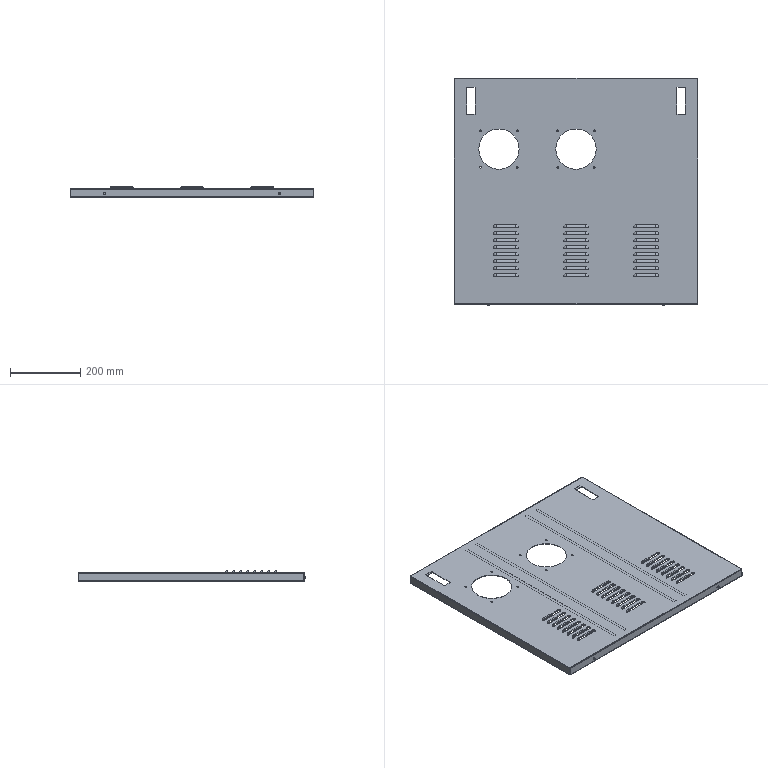Part | STEP file | FBDS-BJ-004 | 3 solids | 548 faces | box 695 x 650 x 31 mm | volume 909135 mm3 | plane 182 | cylinder 156 | torus 96 | sphere 96 | spline 16 | cone 2 | commonest cylinder face diameters 1 x24 4 x24 12 x24 15 x24 0.4 x16 3.4 x16